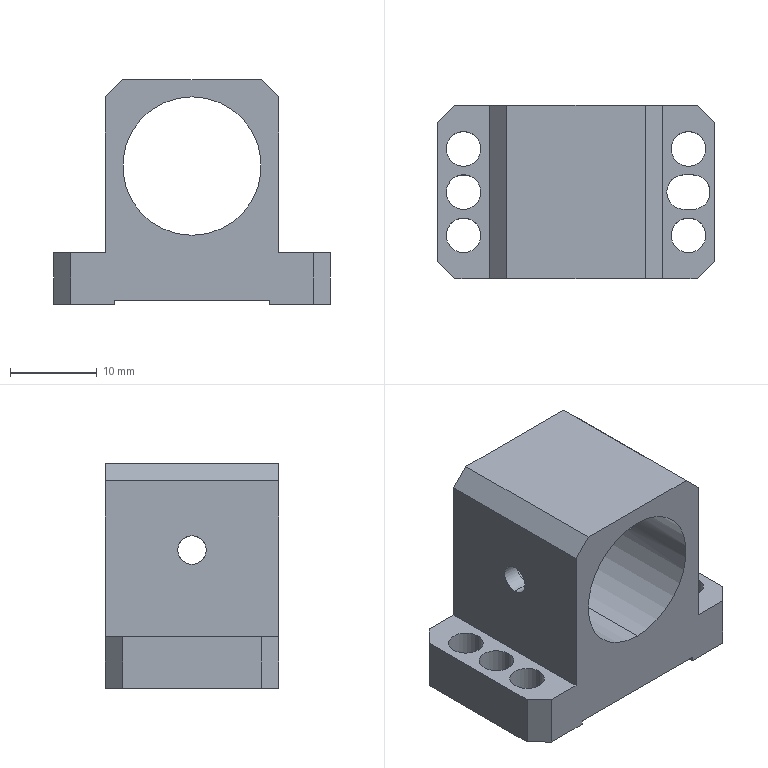NC program | NX | posted with a generic post | part box 32 x 20 x 26 mm
Whole program:
N10 G17 G21 G94 G90
(HOLE_MILLING , TOOL : D10)
N12 T10 M6
N14 G54
N16 G17 G0 G90 X0. Y-3. B0. C0. S9500 M3
N18 G43 Z30. H10
N20 Z0.5
N22 G94 G3 X1.45 Y-4.45 R1.45 F2000.
N24 X2.9 Y-3. R1.45
N26 X2.9 Y-3. Z0. I-2.9 J0.
N28 X2.9 Y-3. Z-0.5 I-2.9 J0.
N30 X2.9 Y-3. Z-1. I-2.9 J0.
N32 X2.9 Y-3. Z-1.5 I-2.9 J0.
N34 X2.9 Y-3. Z-2. I-2.9 J0.
N36 X2.9 Y-3. Z-2.5 I-2.9 J0.
N38 X2.9 Y-3. Z-3. I-2.9 J0.
N40 X2.9 Y-3. Z-3.5 I-2.9 J0.
N42 X2.9 Y-3. Z-4. I-2.9 J0.
N44 X2.9 Y-3. Z-4.5 I-2.9 J0.
N46 X2.9 Y-3. Z-5. I-2.9 J0.
N48 X2.9 Y-3. Z-5.5 I-2.9 J0.
N50 X2.9 Y-3. Z-6. I-2.9 J0.
N52 X2.9 Y-3. Z-6.5 I-2.9 J0.
N54 X2.9 Y-3. Z-7. I-2.9 J0.
N56 X2.9 Y-3. Z-7.5 I-2.9 J0.
N58 X2.9 Y-3. Z-8. I-2.9 J0.
N60 X2.9 Y-3. Z-8.5 I-2.9 J0.
N62 X2.9 Y-3. Z-9. I-2.9 J0.
N64 X2.9 Y-3. Z-9.5 I-2.9 J0.
N66 X2.9 Y-3. Z-10. I-2.9 J0.
N68 X2.9 Y-3. Z-10.5 I-2.9 J0.
N70 X2.9 Y-3. Z-11. I-2.9 J0.
N72 X2.9 Y-3. Z-11.5 I-2.9 J0.
N74 X2.9 Y-3. Z-12. I-2.9 J0.
N76 X2.9 Y-3. Z-12.5 I-2.9 J0.
N78 X2.9 Y-3. Z-13. I-2.9 J0.
N80 X2.9 Y-3. Z-13.5 I-2.9 J0.
N82 X2.9 Y-3. Z-14. I-2.9 J0.
N84 X2.9 Y-3. Z-14.5 I-2.9 J0.
N86 X2.9 Y-3. Z-15. I-2.9 J0.
N88 X2.9 Y-3. Z-15.5 I-2.9 J0.
N90 X2.9 Y-3. Z-16. I-2.9 J0.
N92 X2.9 Y-3. Z-16.5 I-2.9 J0.
N94 X2.9 Y-3. Z-17. I-2.9 J0.
N96 X2.9 Y-3. Z-17.5 I-2.9 J0.
N98 X2.9 Y-3. Z-18. I-2.9 J0.
N100 X2.9 Y-3. Z-18.5 I-2.9 J0.
N102 X2.9 Y-3. Z-19. I-2.9 J0.
N104 X2.9 Y-3. Z-19.5 I-2.9 J0.
N106 X2.9 Y-3. Z-20. I-2.9 J0.
N108 X0. Y-0.1 R2.9
N110 X2.9 Y-3. R-2.9
N112 X1.45 Y-1.55 R1.45
N114 X0. Y-3. R1.45
N116 G0 Z30.
N118 M5
(PLANAR_MILL_COPY_COPY_1_COPY_COPY_COPY , TOOL : D6A45)
N120 T07 M6
N122 G54
N124 G17 G0 G90 X-1.36 Y-8.844 B0. C0. S9500 M3
N126 G43 Z30. H7
N128 Z0.5
N130 G94 G1 Z-1. F1250.
N132 X-0.866 Y-9.7
N134 G3 X0. Y-10.2 R1.
N136 X7.2 Y-3. R7.2
N138 X0. Y-10.2 R-7.2
N140 X0.866 Y-9.7 R1.
N142 G1 X1.36 Y-8.844
N144 Z0.5
N146 G0 Z30.
N148 M5
(刀补 , TOOL : D10JING)
N150 T11 M6
N152 G54
N154 G17 G0 G90 X0. Y-3. B0. C0. S9500 M3
N156 G43 Z30. H11
N158 Z0.5
N160 G41 G94 G1 X-0.011 Y-3.099 F1000. D11
N162 G3 X2.95 Y-3. R1.482
N164 X2.95 Y-3. Z-4.5 I-2.95 J0.
N166 X2.95 Y-3. Z-9.5 I-2.95 J0.
N168 X2.95 Y-3. Z-14.5 I-2.95 J0.
N170 X2.95 Y-3. Z-19.5 I-2.95 J0.
N172 X2.387 Y-1.266 Z-20. R2.95
N174 X-1.734 Y-0.613 R2.95
N176 X2.387 Y-1.266 R-2.95
N178 X-0.067 Y-2.926 R1.482
N180 G40
N182 G1 X0. Y-3.
N184 G0 Z30.
N186 M5
N188 M2